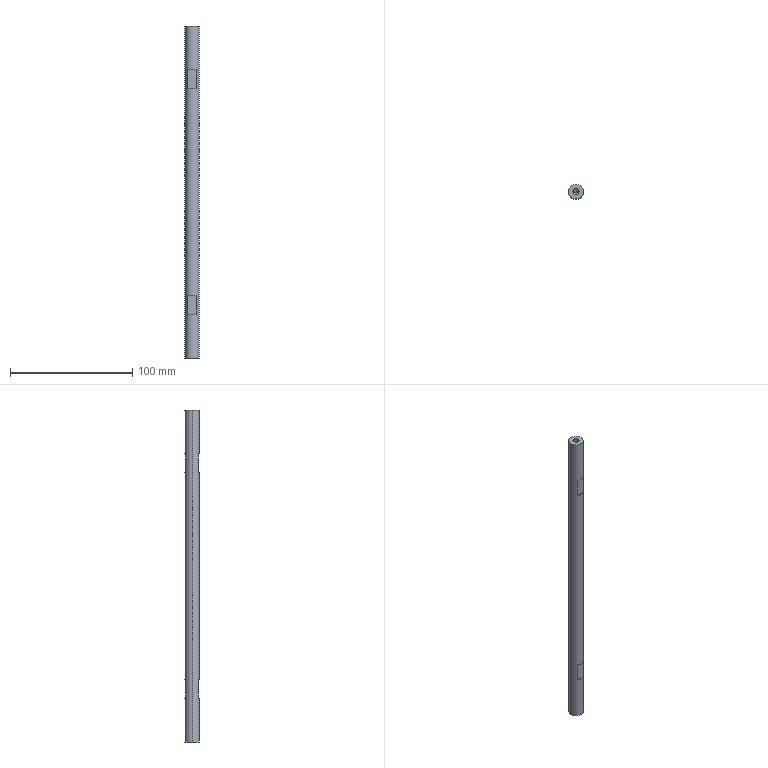Part | STEP file | GLSJ-10-30_default | 1 solid | 24 faces | box 12 x 12 x 272 mm | volume 29884 mm3 | plane 14 | cylinder 6 | cone 4 | commonest cylinder face diameters 5 x4 12 x2
STEP:
#1=CARTESIAN_POINT('',(0.,0.,0.));
#2=DIRECTION('',(0.,0.,1.));
#3=DIRECTION('',(1.,0.,0.));
#4=AXIS2_PLACEMENT_3D('',#1,#2,#3);
#5=CARTESIAN_POINT('',(-2.5,0.,-121.));
#6=VERTEX_POINT('',#5);
#7=CARTESIAN_POINT('',(-2.5,0.,-136.));
#8=VERTEX_POINT('',#7);
#9=CARTESIAN_POINT('',(-2.5,0.,-136.));
#10=DIRECTION('',(0.,0.,-1.));
#11=VECTOR('',#10,1.);
#12=LINE('',#9,#11);
#13=CARTESIAN_POINT('',(0.,0.,-136.));
#14=DIRECTION('',(0.,0.,-1.));
#15=DIRECTION('',(-1.,0.,0.));
#16=AXIS2_PLACEMENT_3D('',#13,#14,#15);
#17=CYLINDRICAL_SURFACE('',#16,2.5);
#18=CARTESIAN_POINT('',(6.283,0.));
#19=DIRECTION('',(0.,1.));
#20=VECTOR('',#19,1.);
#21=LINE('',#18,#20);
#22=(GEOMETRIC_REPRESENTATION_CONTEXT(2)PARAMETRIC_REPRESENTATION_CONTEXT()REPRESENTATION_CONTEXT('',''));
#23=DEFINITIONAL_REPRESENTATION('',(#21),#22);
#24=PCURVE('',#17,#23);
#25=CARTESIAN_POINT('',(0.,0.,-136.));
#26=DIRECTION('',(0.,0.,-1.));
#27=DIRECTION('',(-1.,0.,0.));
#28=AXIS2_PLACEMENT_3D('',#25,#26,#27);
#29=CYLINDRICAL_SURFACE('',#28,2.5);
#30=CARTESIAN_POINT('',(0.,0.));
#31=DIRECTION('',(0.,1.));
#32=VECTOR('',#31,1.);
#33=LINE('',#30,#32);
#34=(GEOMETRIC_REPRESENTATION_CONTEXT(2)PARAMETRIC_REPRESENTATION_CONTEXT()REPRESENTATION_CONTEXT('',''));
#35=DEFINITIONAL_REPRESENTATION('',(#33),#34);
#36=PCURVE('',#29,#35);
#37=SURFACE_CURVE('',#12,(#24,#36),.PCURVE_S1.);
#38=EDGE_CURVE('',#6,#8,#37,.T.);
#39=ORIENTED_EDGE('',*,*,#38,.T.);
#40=CARTESIAN_POINT('',(2.5,0.,-136.));
#41=VERTEX_POINT('',#40);
#42=CARTESIAN_POINT('',(0.,0.,-136.));
#43=DIRECTION('',(0.,0.,-1.));
#44=DIRECTION('',(-1.,0.,0.));
#45=AXIS2_PLACEMENT_3D('',#42,#43,#44);
#46=CIRCLE('',#45,2.5);
#47=CARTESIAN_POINT('',(0.,0.));
#48=DIRECTION('',(1.,0.));
#49=VECTOR('',#48,1.);
#50=LINE('',#47,#49);
#51=(GEOMETRIC_REPRESENTATION_CONTEXT(2)PARAMETRIC_REPRESENTATION_CONTEXT()REPRESENTATION_CONTEXT('',''));
#52=DEFINITIONAL_REPRESENTATION('',(#50),#51);
#53=PCURVE('',#17,#52);
#54=CARTESIAN_POINT('',(0.,0.,-136.));
#55=DIRECTION('',(0.,0.,1.));
#56=DIRECTION('',(1.,0.,0.));
#57=AXIS2_PLACEMENT_3D('',#54,#55,#56);
#58=PLANE('',#57);
#59=CARTESIAN_POINT('',(-2.5,0.));
#60=CARTESIAN_POINT('',(-2.5,4.33));
#61=CARTESIAN_POINT('',(1.25,2.165));
#62=CARTESIAN_POINT('',(5.,0.));
#63=CARTESIAN_POINT('',(1.25,-2.165));
#64=CARTESIAN_POINT('',(-2.5,-4.33));
#65=CARTESIAN_POINT('',(-2.5,0.));
#66=(BOUNDED_CURVE()B_SPLINE_CURVE(2,(#59,#60,#61,#62,#63,#64,#65),.UNSPECIFIED.,.T.,.F.)B_SPLINE_CURVE_WITH_KNOTS((1,2,2,2,2,1),(-2.094,0.,2.094,4.189,6.283,8.378),.UNSPECIFIED.)CURVE()GEOMETRIC_REPRESENTATION_ITEM()RATIONAL_B_SPLINE_CURVE((1.,0.5,1.,0.5,1.,0.5,1.))REPRESENTATION_ITEM(''));
#67=(GEOMETRIC_REPRESENTATION_CONTEXT(2)PARAMETRIC_REPRESENTATION_CONTEXT()REPRESENTATION_CONTEXT('',''));
#68=DEFINITIONAL_REPRESENTATION('',(#66),#67);
#69=PCURVE('',#58,#68);
#70=SURFACE_CURVE('',#46,(#53,#69),.PCURVE_S1.);
#71=EDGE_CURVE('',#41,#8,#70,.T.);
#72=ORIENTED_EDGE('',*,*,#71,.F.);
#73=CARTESIAN_POINT('',(2.5,0.,-121.));
#74=VERTEX_POINT('',#73);
#75=CARTESIAN_POINT('',(2.5,0.,-136.));
#76=DIRECTION('',(0.,0.,-1.));
#77=VECTOR('',#76,1.);
#78=LINE('',#75,#77);
#79=CARTESIAN_POINT('',(3.142,0.));
#80=DIRECTION('',(0.,1.));
#81=VECTOR('',#80,1.);
#82=LINE('',#79,#81);
#83=(GEOMETRIC_REPRESENTATION_CONTEXT(2)PARAMETRIC_REPRESENTATION_CONTEXT()REPRESENTATION_CONTEXT('',''));
#84=DEFINITIONAL_REPRESENTATION('',(#82),#83);
#85=PCURVE('',#17,#84);
#86=CARTESIAN_POINT('',(3.142,0.));
#87=DIRECTION('',(0.,1.));
#88=VECTOR('',#87,1.);
#89=LINE('',#86,#88);
#90=(GEOMETRIC_REPRESENTATION_CONTEXT(2)PARAMETRIC_REPRESENTATION_CONTEXT()REPRESENTATION_CONTEXT('',''));
#91=DEFINITIONAL_REPRESENTATION('',(#89),#90);
#92=PCURVE('',#29,#91);
#93=SURFACE_CURVE('',#78,(#85,#92),.PCURVE_S1.);
#94=EDGE_CURVE('',#74,#41,#93,.T.);
#95=ORIENTED_EDGE('',*,*,#94,.F.);
#96=CARTESIAN_POINT('',(0.,0.,-121.));
#97=DIRECTION('',(0.,0.,-1.));
#98=DIRECTION('',(-1.,0.,0.));
#99=AXIS2_PLACEMENT_3D('',#96,#97,#98);
#100=CIRCLE('',#99,2.5);
#101=CARTESIAN_POINT('',(0.,-15.));
#102=DIRECTION('',(1.,0.));
#103=VECTOR('',#102,1.);
#104=LINE('',#101,#103);
#105=(GEOMETRIC_REPRESENTATION_CONTEXT(2)PARAMETRIC_REPRESENTATION_CONTEXT()REPRESENTATION_CONTEXT('',''));
#106=DEFINITIONAL_REPRESENTATION('',(#104),#105);
#107=PCURVE('',#17,#106);
#108=CARTESIAN_POINT('',(0.,0.,-121.));
#109=DIRECTION('',(0.,0.,-1.));
#110=DIRECTION('',(-1.,0.,0.));
#111=AXIS2_PLACEMENT_3D('',#108,#109,#110);
#112=CONICAL_SURFACE('',#111,2.5,1.03);
#113=CARTESIAN_POINT('',(0.,0.));
#114=DIRECTION('',(1.,0.));
#115=VECTOR('',#114,1.);
#116=LINE('',#113,#115);
#117=(GEOMETRIC_REPRESENTATION_CONTEXT(2)PARAMETRIC_REPRESENTATION_CONTEXT()REPRESENTATION_CONTEXT('',''));
#118=DEFINITIONAL_REPRESENTATION('',(#116),#117);
#119=PCURVE('',#112,#118);
#120=SURFACE_CURVE('',#100,(#107,#119),.PCURVE_S1.);
#121=EDGE_CURVE('',#74,#6,#120,.T.);
#122=ORIENTED_EDGE('',*,*,#121,.T.);
#123=EDGE_LOOP('',(#39,#72,#95,#122));
#124=FACE_BOUND('',#123,.F.);
#125=ADVANCED_FACE('',(#124),#17,.F.);
#126=ORIENTED_EDGE('',*,*,#121,.F.);
#127=CARTESIAN_POINT('',(0.,0.,-119.498));
#128=VERTEX_POINT('',#127);
#129=CARTESIAN_POINT('',(2.5,0.,-121.));
#130=DIRECTION('',(0.8572,0.,-0.515));
#131=VECTOR('',#130,1.);
#132=LINE('',#129,#131);
#133=CARTESIAN_POINT('',(3.142,-1.502));
#134=CARTESIAN_POINT('',(3.142,-1.479));
#135=CARTESIAN_POINT('',(3.142,-1.434));
#136=CARTESIAN_POINT('',(3.142,-1.366));
#137=CARTESIAN_POINT('',(3.142,-1.297));
#138=CARTESIAN_POINT('',(3.142,-1.229));
#139=CARTESIAN_POINT('',(3.142,-1.161));
#140=CARTESIAN_POINT('',(3.142,-1.092));
#141=CARTESIAN_POINT('',(3.142,-1.024));
#142=CARTESIAN_POINT('',(3.142,-0.9559));
#143=CARTESIAN_POINT('',(3.142,-0.8876));
#144=CARTESIAN_POINT('',(3.142,-0.8194));
#145=CARTESIAN_POINT('',(3.142,-0.7511));
#146=CARTESIAN_POINT('',(3.142,-0.6828));
#147=CARTESIAN_POINT('',(3.142,-0.6145));
#148=CARTESIAN_POINT('',(3.142,-0.5462));
#149=CARTESIAN_POINT('',(3.142,-0.478));
#150=CARTESIAN_POINT('',(3.142,-0.4097));
#151=CARTESIAN_POINT('',(3.142,-0.3414));
#152=CARTESIAN_POINT('',(3.142,-0.2731));
#153=CARTESIAN_POINT('',(3.142,-0.2048));
#154=CARTESIAN_POINT('',(3.142,-0.1366));
#155=CARTESIAN_POINT('',(3.142,-0.06828));
#156=CARTESIAN_POINT('',(3.142,-0.02276));
#157=CARTESIAN_POINT('',(3.142,0.));
#158=B_SPLINE_CURVE_WITH_KNOTS('',3,(#133,#134,#135,#136,#137,#138,#139,#140,#141,#142,#143,#144,#145,#146,#147,#148,#149,#150,#151,#152,#153,#154,#155,#156,#157),.UNSPECIFIED.,.F.,.F.,(4,1,1,1,1,1,1,1,1,1,1,1,1,1,1,1,1,1,1,1,1,1,4),(-2.917,-2.784,-2.651,-2.519,-2.386,-2.254,-2.121,-1.989,-1.856,-1.723,-1.591,-1.458,-1.326,-1.193,-1.061,-0.928,-0.7954,-0.6629,-0.5303,-0.3977,-0.2651,-0.1326,0.),.QUASI_UNIFORM_KNOTS.);
#159=(GEOMETRIC_REPRESENTATION_CONTEXT(2)PARAMETRIC_REPRESENTATION_CONTEXT()REPRESENTATION_CONTEXT('',''));
#160=DEFINITIONAL_REPRESENTATION('',(#158),#159);
#161=PCURVE('',#112,#160);
#162=CARTESIAN_POINT('',(0.,0.,-121.));
#163=DIRECTION('',(0.,0.,-1.));
#164=DIRECTION('',(-1.,0.,0.));
#165=AXIS2_PLACEMENT_3D('',#162,#163,#164);
#166=CONICAL_SURFACE('',#165,2.5,1.03);
#167=CARTESIAN_POINT('',(3.142,-1.502));
#168=CARTESIAN_POINT('',(3.142,-1.479));
#169=CARTESIAN_POINT('',(3.142,-1.434));
#170=CARTESIAN_POINT('',(3.142,-1.366));
#171=CARTESIAN_POINT('',(3.142,-1.297));
#172=CARTESIAN_POINT('',(3.142,-1.229));
#173=CARTESIAN_POINT('',(3.142,-1.161));
#174=CARTESIAN_POINT('',(3.142,-1.092));
#175=CARTESIAN_POINT('',(3.142,-1.024));
#176=CARTESIAN_POINT('',(3.142,-0.9559));
#177=CARTESIAN_POINT('',(3.142,-0.8876));
#178=CARTESIAN_POINT('',(3.142,-0.8194));
#179=CARTESIAN_POINT('',(3.142,-0.7511));
#180=CARTESIAN_POINT('',(3.142,-0.6828));
#181=CARTESIAN_POINT('',(3.142,-0.6145));
#182=CARTESIAN_POINT('',(3.142,-0.5462));
#183=CARTESIAN_POINT('',(3.142,-0.478));
#184=CARTESIAN_POINT('',(3.142,-0.4097));
#185=CARTESIAN_POINT('',(3.142,-0.3414));
#186=CARTESIAN_POINT('',(3.142,-0.2731));
#187=CARTESIAN_POINT('',(3.142,-0.2048));
#188=CARTESIAN_POINT('',(3.142,-0.1366));
#189=CARTESIAN_POINT('',(3.142,-0.06828));
#190=CARTESIAN_POINT('',(3.142,-0.02276));
#191=CARTESIAN_POINT('',(3.142,0.));
#192=B_SPLINE_CURVE_WITH_KNOTS('',3,(#167,#168,#169,#170,#171,#172,#173,#174,#175,#176,#177,#178,#179,#180,#181,#182,#183,#184,#185,#186,#187,#188,#189,#190,#191),.UNSPECIFIED.,.F.,.F.,(4,1,1,1,1,1,1,1,1,1,1,1,1,1,1,1,1,1,1,1,1,1,4),(-2.917,-2.784,-2.651,-2.519,-2.386,-2.254,-2.121,-1.989,-1.856,-1.723,-1.591,-1.458,-1.326,-1.193,-1.061,-0.928,-0.7954,-0.6629,-0.5303,-0.3977,-0.2651,-0.1326,0.),.QUASI_UNIFORM_KNOTS.);
#193=(GEOMETRIC_REPRESENTATION_CONTEXT(2)PARAMETRIC_REPRESENTATION_CONTEXT()REPRESENTATION_CONTEXT('',''));
#194=DEFINITIONAL_REPRESENTATION('',(#192),#193);
#195=PCURVE('',#166,#194);
#196=SURFACE_CURVE('',#132,(#161,#195),.PCURVE_S1.);
#197=EDGE_CURVE('',#128,#74,#196,.T.);
#198=ORIENTED_EDGE('',*,*,#197,.F.);
#199=CARTESIAN_POINT('',(-2.5,0.,-121.));
#200=DIRECTION('',(-0.8572,0.,-0.515));
#201=VECTOR('',#200,1.);
#202=LINE('',#199,#201);
#203=CARTESIAN_POINT('',(6.283,0.));
#204=DIRECTION('',(0.,1.));
#205=VECTOR('',#204,1.);
#206=LINE('',#203,#205);
#207=(GEOMETRIC_REPRESENTATION_CONTEXT(2)PARAMETRIC_REPRESENTATION_CONTEXT()REPRESENTATION_CONTEXT('',''));
#208=DEFINITIONAL_REPRESENTATION('',(#206),#207);
#209=PCURVE('',#112,#208);
#210=CARTESIAN_POINT('',(0.,0.));
#211=DIRECTION('',(0.,1.));
#212=VECTOR('',#211,1.);
#213=LINE('',#210,#212);
#214=(GEOMETRIC_REPRESENTATION_CONTEXT(2)PARAMETRIC_REPRESENTATION_CONTEXT()REPRESENTATION_CONTEXT('',''));
#215=DEFINITIONAL_REPRESENTATION('',(#213),#214);
#216=PCURVE('',#166,#215);
#217=SURFACE_CURVE('',#202,(#209,#216),.PCURVE_S1.);
#218=EDGE_CURVE('',#128,#6,#217,.T.);
#219=ORIENTED_EDGE('',*,*,#218,.T.);
#220=EDGE_LOOP('',(#126,#198,#219));
#221=FACE_BOUND('',#220,.F.);
#222=ADVANCED_FACE('',(#221),#112,.F.);
#223=CARTESIAN_POINT('',(2.5,0.,121.));
#224=VERTEX_POINT('',#223);
#225=CARTESIAN_POINT('',(2.5,0.,136.));
#226=VERTEX_POINT('',#225);
#227=CARTESIAN_POINT('',(2.5,0.,136.));
#228=DIRECTION('',(0.,0.,1.));
#229=VECTOR('',#228,1.);
#230=LINE('',#227,#229);
#231=CARTESIAN_POINT('',(0.,0.,136.));
#232=DIRECTION('',(0.,0.,1.));
#233=DIRECTION('',(1.,0.,0.));
#234=AXIS2_PLACEMENT_3D('',#231,#232,#233);
#235=CYLINDRICAL_SURFACE('',#234,2.5);
#236=CARTESIAN_POINT('',(6.283,0.));
#237=DIRECTION('',(0.,1.));
#238=VECTOR('',#237,1.);
#239=LINE('',#236,#238);
#240=(GEOMETRIC_REPRESENTATION_CONTEXT(2)PARAMETRIC_REPRESENTATION_CONTEXT()REPRESENTATION_CONTEXT('',''));
#241=DEFINITIONAL_REPRESENTATION('',(#239),#240);
#242=PCURVE('',#235,#241);
#243=CARTESIAN_POINT('',(0.,0.,136.));
#244=DIRECTION('',(0.,0.,1.));
#245=DIRECTION('',(1.,0.,0.));
#246=AXIS2_PLACEMENT_3D('',#243,#244,#245);
#247=CYLINDRICAL_SURFACE('',#246,2.5);
#248=CARTESIAN_POINT('',(0.,0.));
#249=DIRECTION('',(0.,1.));
#250=VECTOR('',#249,1.);
#251=LINE('',#248,#250);
#252=(GEOMETRIC_REPRESENTATION_CONTEXT(2)PARAMETRIC_REPRESENTATION_CONTEXT()REPRESENTATION_CONTEXT('',''));
#253=DEFINITIONAL_REPRESENTATION('',(#251),#252);
#254=PCURVE('',#247,#253);
#255=SURFACE_CURVE('',#230,(#242,#254),.PCURVE_S1.);
#256=EDGE_CURVE('',#224,#226,#255,.T.);
#257=ORIENTED_EDGE('',*,*,#256,.T.);
#258=CARTESIAN_POINT('',(-2.5,0.,136.));
#259=VERTEX_POINT('',#258);
#260=CARTESIAN_POINT('',(0.,0.,136.));
#261=DIRECTION('',(0.,0.,1.));
#262=DIRECTION('',(1.,0.,0.));
#263=AXIS2_PLACEMENT_3D('',#260,#261,#262);
#264=CIRCLE('',#263,2.5);
#265=CARTESIAN_POINT('',(0.,0.));
#266=DIRECTION('',(1.,0.));
#267=VECTOR('',#266,1.);
#268=LINE('',#265,#267);
#269=(GEOMETRIC_REPRESENTATION_CONTEXT(2)PARAMETRIC_REPRESENTATION_CONTEXT()REPRESENTATION_CONTEXT('',''));
#270=DEFINITIONAL_REPRESENTATION('',(#268),#269);
#271=PCURVE('',#235,#270);
#272=CARTESIAN_POINT('',(0.,0.,136.));
#273=DIRECTION('',(0.,0.,1.));
#274=DIRECTION('',(1.,0.,0.));
#275=AXIS2_PLACEMENT_3D('',#272,#273,#274);
#276=PLANE('',#275);
#277=CARTESIAN_POINT('',(0.,0.));
#278=DIRECTION('',(1.,0.));
#279=AXIS2_PLACEMENT_2D('',#277,#278);
#280=CIRCLE('',#279,2.5);
#281=(GEOMETRIC_REPRESENTATION_CONTEXT(2)PARAMETRIC_REPRESENTATION_CONTEXT()REPRESENTATION_CONTEXT('',''));
#282=DEFINITIONAL_REPRESENTATION('',(#280),#281);
#283=PCURVE('',#276,#282);
#284=SURFACE_CURVE('',#264,(#271,#283),.PCURVE_S1.);
#285=EDGE_CURVE('',#259,#226,#284,.T.);
#286=ORIENTED_EDGE('',*,*,#285,.F.);
#287=CARTESIAN_POINT('',(-2.5,0.,121.));
#288=VERTEX_POINT('',#287);
#289=CARTESIAN_POINT('',(-2.5,0.,136.));
#290=DIRECTION('',(0.,0.,1.));
#291=VECTOR('',#290,1.);
#292=LINE('',#289,#291);
#293=CARTESIAN_POINT('',(3.142,0.));
#294=DIRECTION('',(0.,1.));
#295=VECTOR('',#294,1.);
#296=LINE('',#293,#295);
#297=(GEOMETRIC_REPRESENTATION_CONTEXT(2)PARAMETRIC_REPRESENTATION_CONTEXT()REPRESENTATION_CONTEXT('',''));
#298=DEFINITIONAL_REPRESENTATION('',(#296),#297);
#299=PCURVE('',#235,#298);
#300=CARTESIAN_POINT('',(3.142,0.));
#301=DIRECTION('',(0.,1.));
#302=VECTOR('',#301,1.);
#303=LINE('',#300,#302);
#304=(GEOMETRIC_REPRESENTATION_CONTEXT(2)PARAMETRIC_REPRESENTATION_CONTEXT()REPRESENTATION_CONTEXT('',''));
#305=DEFINITIONAL_REPRESENTATION('',(#303),#304);
#306=PCURVE('',#247,#305);
#307=SURFACE_CURVE('',#292,(#299,#306),.PCURVE_S1.);
#308=EDGE_CURVE('',#288,#259,#307,.T.);
#309=ORIENTED_EDGE('',*,*,#308,.F.);
#310=CARTESIAN_POINT('',(0.,0.,121.));
#311=DIRECTION('',(0.,0.,1.));
#312=DIRECTION('',(1.,0.,0.));
#313=AXIS2_PLACEMENT_3D('',#310,#311,#312);
#314=CIRCLE('',#313,2.5);
#315=CARTESIAN_POINT('',(0.,-15.));
#316=DIRECTION('',(1.,0.));
#317=VECTOR('',#316,1.);
#318=LINE('',#315,#317);
#319=(GEOMETRIC_REPRESENTATION_CONTEXT(2)PARAMETRIC_REPRESENTATION_CONTEXT()REPRESENTATION_CONTEXT('',''));
#320=DEFINITIONAL_REPRESENTATION('',(#318),#319);
#321=PCURVE('',#235,#320);
#322=CARTESIAN_POINT('',(0.,0.,121.));
#323=DIRECTION('',(0.,0.,1.));
#324=DIRECTION('',(1.,0.,0.));
#325=AXIS2_PLACEMENT_3D('',#322,#323,#324);
#326=CONICAL_SURFACE('',#325,2.5,1.03);
#327=CARTESIAN_POINT('',(0.,0.));
#328=DIRECTION('',(1.,0.));
#329=VECTOR('',#328,1.);
#330=LINE('',#327,#329);
#331=(GEOMETRIC_REPRESENTATION_CONTEXT(2)PARAMETRIC_REPRESENTATION_CONTEXT()REPRESENTATION_CONTEXT('',''));
#332=DEFINITIONAL_REPRESENTATION('',(#330),#331);
#333=PCURVE('',#326,#332);
#334=SURFACE_CURVE('',#314,(#321,#333),.PCURVE_S1.);
#335=EDGE_CURVE('',#288,#224,#334,.T.);
#336=ORIENTED_EDGE('',*,*,#335,.T.);
#337=EDGE_LOOP('',(#257,#286,#309,#336));
#338=FACE_BOUND('',#337,.F.);
#339=ADVANCED_FACE('',(#338),#235,.F.);
#340=ORIENTED_EDGE('',*,*,#335,.F.);
#341=CARTESIAN_POINT('',(0.,0.,119.498));
#342=VERTEX_POINT('',#341);
#343=CARTESIAN_POINT('',(-2.5,0.,121.));
#344=DIRECTION('',(-0.8572,0.,0.515));
#345=VECTOR('',#344,1.);
#346=LINE('',#343,#345);
#347=CARTESIAN_POINT('',(3.142,0.));
#348=DIRECTION('',(0.,1.));
#349=VECTOR('',#348,1.);
#350=LINE('',#347,#349);
#351=(GEOMETRIC_REPRESENTATION_CONTEXT(2)PARAMETRIC_REPRESENTATION_CONTEXT()REPRESENTATION_CONTEXT('',''));
#352=DEFINITIONAL_REPRESENTATION('',(#350),#351);
#353=PCURVE('',#326,#352);
#354=CARTESIAN_POINT('',(0.,0.,121.));
#355=DIRECTION('',(0.,0.,1.));
#356=DIRECTION('',(1.,0.,0.));
#357=AXIS2_PLACEMENT_3D('',#354,#355,#356);
#358=CONICAL_SURFACE('',#357,2.5,1.03);
#359=CARTESIAN_POINT('',(3.142,0.));
#360=DIRECTION('',(0.,1.));
#361=VECTOR('',#360,1.);
#362=LINE('',#359,#361);
#363=(GEOMETRIC_REPRESENTATION_CONTEXT(2)PARAMETRIC_REPRESENTATION_CONTEXT()REPRESENTATION_CONTEXT('',''));
#364=DEFINITIONAL_REPRESENTATION('',(#362),#363);
#365=PCURVE('',#358,#364);
#366=SURFACE_CURVE('',#346,(#353,#365),.PCURVE_S1.);
#367=EDGE_CURVE('',#342,#288,#366,.T.);
#368=ORIENTED_EDGE('',*,*,#367,.F.);
#369=CARTESIAN_POINT('',(2.5,0.,121.));
#370=DIRECTION('',(0.8572,0.,0.515));
#371=VECTOR('',#370,1.);
#372=LINE('',#369,#371);
#373=CARTESIAN_POINT('',(6.283,-1.502));
#374=CARTESIAN_POINT('',(6.283,-1.479));
#375=CARTESIAN_POINT('',(6.283,-1.434));
#376=CARTESIAN_POINT('',(6.283,-1.366));
#377=CARTESIAN_POINT('',(6.283,-1.297));
#378=CARTESIAN_POINT('',(6.283,-1.229));
#379=CARTESIAN_POINT('',(6.283,-1.161));
#380=CARTESIAN_POINT('',(6.283,-1.092));
#381=CARTESIAN_POINT('',(6.283,-1.024));
#382=CARTESIAN_POINT('',(6.283,-0.9559));
#383=CARTESIAN_POINT('',(6.283,-0.8876));
#384=CARTESIAN_POINT('',(6.283,-0.8194));
#385=CARTESIAN_POINT('',(6.283,-0.7511));
#386=CARTESIAN_POINT('',(6.283,-0.6828));
#387=CARTESIAN_POINT('',(6.283,-0.6145));
#388=CARTESIAN_POINT('',(6.283,-0.5462));
#389=CARTESIAN_POINT('',(6.283,-0.478));
#390=CARTESIAN_POINT('',(6.283,-0.4097));
#391=CARTESIAN_POINT('',(6.283,-0.3414));
#392=CARTESIAN_POINT('',(6.283,-0.2731));
#393=CARTESIAN_POINT('',(6.283,-0.2048));
#394=CARTESIAN_POINT('',(6.283,-0.1366));
#395=CARTESIAN_POINT('',(6.283,-0.06828));
#396=CARTESIAN_POINT('',(6.283,-0.02276));
#397=CARTESIAN_POINT('',(6.283,0.));
#398=B_SPLINE_CURVE_WITH_KNOTS('',3,(#373,#374,#375,#376,#377,#378,#379,#380,#381,#382,#383,#384,#385,#386,#387,#388,#389,#390,#391,#392,#393,#394,#395,#396,#397),.UNSPECIFIED.,.F.,.F.,(4,1,1,1,1,1,1,1,1,1,1,1,1,1,1,1,1,1,1,1,1,1,4),(-2.917,-2.784,-2.651,-2.519,-2.386,-2.254,-2.121,-1.989,-1.856,-1.723,-1.591,-1.458,-1.326,-1.193,-1.061,-0.928,-0.7954,-0.6629,-0.5303,-0.3977,-0.2651,-0.1326,0.),.QUASI_UNIFORM_KNOTS.);
#399=(GEOMETRIC_REPRESENTATION_CONTEXT(2)PARAMETRIC_REPRESENTATION_CONTEXT()REPRESENTATION_CONTEXT('',''));
#400=DEFINITIONAL_REPRESENTATION('',(#398),#399);
#401=PCURVE('',#326,#400);
#402=CARTESIAN_POINT('',(0.,-1.502));
#403=CARTESIAN_POINT('',(0.,-1.479));
#404=CARTESIAN_POINT('',(0.,-1.434));
#405=CARTESIAN_POINT('',(0.,-1.366));
#406=CARTESIAN_POINT('',(0.,-1.297));
#407=CARTESIAN_POINT('',(0.,-1.229));
#408=CARTESIAN_POINT('',(0.,-1.161));
#409=CARTESIAN_POINT('',(0.,-1.092));
#410=CARTESIAN_POINT('',(0.,-1.024));
#411=CARTESIAN_POINT('',(0.,-0.9559));
#412=CARTESIAN_POINT('',(0.,-0.8876));
#413=CARTESIAN_POINT('',(0.,-0.8194));
#414=CARTESIAN_POINT('',(0.,-0.7511));
#415=CARTESIAN_POINT('',(0.,-0.6828));
#416=CARTESIAN_POINT('',(0.,-0.6145));
#417=CARTESIAN_POINT('',(0.,-0.5462));
#418=CARTESIAN_POINT('',(0.,-0.478));
#419=CARTESIAN_POINT('',(0.,-0.4097));
#420=CARTESIAN_POINT('',(0.,-0.3414));
#421=CARTESIAN_POINT('',(0.,-0.2731));
#422=CARTESIAN_POINT('',(0.,-0.2048));
#423=CARTESIAN_POINT('',(0.,-0.1366));
#424=CARTESIAN_POINT('',(0.,-0.06828));
#425=CARTESIAN_POINT('',(0.,-0.02276));
#426=CARTESIAN_POINT('',(0.,0.));
#427=B_SPLINE_CURVE_WITH_KNOTS('',3,(#402,#403,#404,#405,#406,#407,#408,#409,#410,#411,#412,#413,#414,#415,#416,#417,#418,#419,#420,#421,#422,#423,#424,#425,#426),.UNSPECIFIED.,.F.,.F.,(4,1,1,1,1,1,1,1,1,1,1,1,1,1,1,1,1,1,1,1,1,1,4),(-2.917,-2.784,-2.651,-2.519,-2.386,-2.254,-2.121,-1.989,-1.856,-1.723,-1.591,-1.458,-1.326,-1.193,-1.061,-0.928,-0.7954,-0.6629,-0.5303,-0.3977,-0.2651,-0.1326,0.),.QUASI_UNIFORM_KNOTS.);
#428=(GEOMETRIC_REPRESENTATION_CONTEXT(2)PARAMETRIC_REPRESENTATION_CONTEXT()REPRESENTATION_CONTEXT('',''));
#429=DEFINITIONAL_REPRESENTATION('',(#427),#428);
#430=PCURVE('',#358,#429);
#431=SURFACE_CURVE('',#372,(#401,#430),.PCURVE_S1.);
#432=EDGE_CURVE('',#342,#224,#431,.T.);
#433=ORIENTED_EDGE('',*,*,#432,.T.);
#434=EDGE_LOOP('',(#340,#368,#433));
#435=FACE_BOUND('',#434,.F.);
#436=ADVANCED_FACE('',(#435),#326,.F.);
#437=CARTESIAN_POINT('',(3.317,5.,100.));
#438=VERTEX_POINT('',#437);
#439=CARTESIAN_POINT('',(-3.317,5.,100.));
#440=VERTEX_POINT('',#439);
#441=CARTESIAN_POINT('',(0.,0.,100.));
#442=DIRECTION('',(0.,0.,1.));
#443=DIRECTION('',(1.,0.,0.));
#444=AXIS2_PLACEMENT_3D('',#441,#442,#443);
#445=CIRCLE('',#444,6.);
#446=CARTESIAN_POINT('',(0.,0.,136.));
#447=DIRECTION('',(0.,0.,-1.));
#448=DIRECTION('',(-1.,0.,0.));
#449=AXIS2_PLACEMENT_3D('',#446,#447,#448);
#450=CYLINDRICAL_SURFACE('',#449,6.);
#451=CARTESIAN_POINT('',(3.142,36.));
#452=DIRECTION('',(-1.,0.));
#453=VECTOR('',#452,1.);
#454=LINE('',#451,#453);
#455=(GEOMETRIC_REPRESENTATION_CONTEXT(2)PARAMETRIC_REPRESENTATION_CONTEXT()REPRESENTATION_CONTEXT('',''));
#456=DEFINITIONAL_REPRESENTATION('',(#454),#455);
#457=PCURVE('',#450,#456);
#458=CARTESIAN_POINT('',(-10.,7.,100.));
#459=DIRECTION('',(0.,0.,1.));
#460=DIRECTION('',(1.,0.,0.));
#461=AXIS2_PLACEMENT_3D('',#458,#459,#460);
#462=PLANE('',#461);
#463=CARTESIAN_POINT('',(10.,-7.));
#464=DIRECTION('',(1.,0.));
#465=AXIS2_PLACEMENT_2D('',#463,#464);
#466=CIRCLE('',#465,6.);
#467=(GEOMETRIC_REPRESENTATION_CONTEXT(2)PARAMETRIC_REPRESENTATION_CONTEXT()REPRESENTATION_CONTEXT('',''));
#468=DEFINITIONAL_REPRESENTATION('',(#466),#467);
#469=PCURVE('',#462,#468);
#470=SURFACE_CURVE('',#445,(#457,#469),.PCURVE_S1.);
#471=EDGE_CURVE('',#438,#440,#470,.T.);
#472=ORIENTED_EDGE('',*,*,#471,.T.);
#473=CARTESIAN_POINT('',(-3.317,5.,85.));
#474=VERTEX_POINT('',#473);
#475=CARTESIAN_POINT('',(-3.317,5.,136.));
#476=DIRECTION('',(0.,0.,-1.));
#477=VECTOR('',#476,1.);
#478=LINE('',#475,#477);
#479=CARTESIAN_POINT('',(0.9851,0.));
#480=DIRECTION('',(0.,1.));
#481=VECTOR('',#480,1.);
#482=LINE('',#479,#481);
#483=(GEOMETRIC_REPRESENTATION_CONTEXT(2)PARAMETRIC_REPRESENTATION_CONTEXT()REPRESENTATION_CONTEXT('',''));
#484=DEFINITIONAL_REPRESENTATION('',(#482),#483);
#485=PCURVE('',#450,#484);
#486=CARTESIAN_POINT('',(-10.,5.,100.));
#487=DIRECTION('',(0.,-1.,0.));
#488=DIRECTION('',(0.,0.,-1.));
#489=AXIS2_PLACEMENT_3D('',#486,#487,#488);
#490=PLANE('',#489);
#491=CARTESIAN_POINT('',(-36.,6.683));
#492=DIRECTION('',(1.,0.));
#493=VECTOR('',#492,1.);
#494=LINE('',#491,#493);
#495=(GEOMETRIC_REPRESENTATION_CONTEXT(2)PARAMETRIC_REPRESENTATION_CONTEXT()REPRESENTATION_CONTEXT('',''));
#496=DEFINITIONAL_REPRESENTATION('',(#494),#495);
#497=PCURVE('',#490,#496);
#498=SURFACE_CURVE('',#478,(#485,#497),.PCURVE_S1.);
#499=EDGE_CURVE('',#440,#474,#498,.T.);
#500=ORIENTED_EDGE('',*,*,#499,.T.);
#501=CARTESIAN_POINT('',(3.317,5.,85.));
#502=VERTEX_POINT('',#501);
#503=CARTESIAN_POINT('',(0.,0.,85.));
#504=DIRECTION('',(0.,0.,-1.));
#505=DIRECTION('',(-1.,0.,0.));
#506=AXIS2_PLACEMENT_3D('',#503,#504,#505);
#507=CIRCLE('',#506,6.);
#508=CARTESIAN_POINT('',(0.,51.));
#509=DIRECTION('',(1.,0.));
#510=VECTOR('',#509,1.);
#511=LINE('',#508,#510);
#512=(GEOMETRIC_REPRESENTATION_CONTEXT(2)PARAMETRIC_REPRESENTATION_CONTEXT()REPRESENTATION_CONTEXT('',''));
#513=DEFINITIONAL_REPRESENTATION('',(#511),#512);
#514=PCURVE('',#450,#513);
#515=CARTESIAN_POINT('',(-10.,7.,85.));
#516=DIRECTION('',(0.,0.,-1.));
#517=DIRECTION('',(-1.,0.,0.));
#518=AXIS2_PLACEMENT_3D('',#515,#516,#517);
#519=PLANE('',#518);
#520=CARTESIAN_POINT('',(-10.,-7.));
#521=DIRECTION('',(1.,0.));
#522=AXIS2_PLACEMENT_2D('',#520,#521);
#523=CIRCLE('',#522,6.);
#524=(GEOMETRIC_REPRESENTATION_CONTEXT(2)PARAMETRIC_REPRESENTATION_CONTEXT()REPRESENTATION_CONTEXT('',''));
#525=DEFINITIONAL_REPRESENTATION('',(#523),#524);
#526=PCURVE('',#519,#525);
#527=SURFACE_CURVE('',#507,(#514,#526),.PCURVE_S1.);
#528=EDGE_CURVE('',#474,#502,#527,.T.);
#529=ORIENTED_EDGE('',*,*,#528,.T.);
#530=CARTESIAN_POINT('',(3.317,5.,136.));
#531=DIRECTION('',(0.,0.,1.));
#532=VECTOR('',#531,1.);
#533=LINE('',#530,#532);
#534=CARTESIAN_POINT('',(2.156,0.));
#535=DIRECTION('',(0.,-1.));
#536=VECTOR('',#535,1.);
#537=LINE('',#534,#536);
#538=(GEOMETRIC_REPRESENTATION_CONTEXT(2)PARAMETRIC_REPRESENTATION_CONTEXT()REPRESENTATION_CONTEXT('',''));
#539=DEFINITIONAL_REPRESENTATION('',(#537),#538);
#540=PCURVE('',#450,#539);
#541=CARTESIAN_POINT('',(-36.,13.317));
#542=DIRECTION('',(-1.,0.));
#543=VECTOR('',#542,1.);
#544=LINE('',#541,#543);
#545=(GEOMETRIC_REPRESENTATION_CONTEXT(2)PARAMETRIC_REPRESENTATION_CONTEXT()REPRESENTATION_CONTEXT('',''));
#546=DEFINITIONAL_REPRESENTATION('',(#544),#545);
#547=PCURVE('',#490,#546);
#548=SURFACE_CURVE('',#533,(#540,#547),.PCURVE_S1.);
#549=EDGE_CURVE('',#502,#438,#548,.T.);
#550=ORIENTED_EDGE('',*,*,#549,.T.);
#551=EDGE_LOOP('',(#472,#500,#529,#550));
#552=FACE_BOUND('',#551,.T.);
#553=CARTESIAN_POINT('',(-3.317,5.,-85.));
#554=VERTEX_POINT('',#553);
#555=CARTESIAN_POINT('',(-3.317,5.,-100.));
#556=VERTEX_POINT('',#555);
#557=CARTESIAN_POINT('',(-3.317,5.,136.));
#558=DIRECTION('',(0.,0.,-1.));
#559=VECTOR('',#558,1.);
#560=LINE('',#557,#559);
#561=CARTESIAN_POINT('',(0.9851,0.));
#562=DIRECTION('',(0.,1.));
#563=VECTOR('',#562,1.);
#564=LINE('',#561,#563);
#565=(GEOMETRIC_REPRESENTATION_CONTEXT(2)PARAMETRIC_REPRESENTATION_CONTEXT()REPRESENTATION_CONTEXT('',''));
#566=DEFINITIONAL_REPRESENTATION('',(#564),#565);
#567=PCURVE('',#450,#566);
#568=CARTESIAN_POINT('',(-10.,5.,-100.));
#569=DIRECTION('',(0.,-1.,0.));
#570=DIRECTION('',(0.,0.,-1.));
#571=AXIS2_PLACEMENT_3D('',#568,#569,#570);
#572=PLANE('',#571);
#573=CARTESIAN_POINT('',(-236.,6.683));
#574=DIRECTION('',(1.,0.));
#575=VECTOR('',#574,1.);
#576=LINE('',#573,#575);
#577=(GEOMETRIC_REPRESENTATION_CONTEXT(2)PARAMETRIC_REPRESENTATION_CONTEXT()REPRESENTATION_CONTEXT('',''));
#578=DEFINITIONAL_REPRESENTATION('',(#576),#577);
#579=PCURVE('',#572,#578);
#580=SURFACE_CURVE('',#560,(#567,#579),.PCURVE_S1.);
#581=EDGE_CURVE('',#554,#556,#580,.T.);
#582=ORIENTED_EDGE('',*,*,#581,.T.);
#583=CARTESIAN_POINT('',(3.317,5.,-100.));
#584=VERTEX_POINT('',#583);
#585=CARTESIAN_POINT('',(0.,0.,-100.));
#586=DIRECTION('',(0.,0.,-1.));
#587=DIRECTION('',(-1.,0.,0.));
#588=AXIS2_PLACEMENT_3D('',#585,#586,#587);
#589=CIRCLE('',#588,6.);
#590=CARTESIAN_POINT('',(0.,236.));
#591=DIRECTION('',(1.,0.));
#592=VECTOR('',#591,1.);
#593=LINE('',#590,#592);
#594=(GEOMETRIC_REPRESENTATION_CONTEXT(2)PARAMETRIC_REPRESENTATION_CONTEXT()REPRESENTATION_CONTEXT('',''));
#595=DEFINITIONAL_REPRESENTATION('',(#593),#594);
#596=PCURVE('',#450,#595);
#597=CARTESIAN_POINT('',(-10.,7.,-100.));
#598=DIRECTION('',(0.,0.,-1.));
#599=DIRECTION('',(-1.,0.,0.));
#600=AXIS2_PLACEMENT_3D('',#597,#598,#599);
#601=PLANE('',#600);
#602=CARTESIAN_POINT('',(-10.,-7.));
#603=DIRECTION('',(1.,0.));
#604=AXIS2_PLACEMENT_2D('',#602,#603);
#605=CIRCLE('',#604,6.);
#606=(GEOMETRIC_REPRESENTATION_CONTEXT(2)PARAMETRIC_REPRESENTATION_CONTEXT()REPRESENTATION_CONTEXT('',''));
#607=DEFINITIONAL_REPRESENTATION('',(#605),#606);
#608=PCURVE('',#601,#607);
#609=SURFACE_CURVE('',#589,(#596,#608),.PCURVE_S1.);
#610=EDGE_CURVE('',#556,#584,#609,.T.);
#611=ORIENTED_EDGE('',*,*,#610,.T.);
#612=CARTESIAN_POINT('',(3.317,5.,-85.));
#613=VERTEX_POINT('',#612);
#614=CARTESIAN_POINT('',(3.317,5.,136.));
#615=DIRECTION('',(0.,0.,1.));
#616=VECTOR('',#615,1.);
#617=LINE('',#614,#616);
#618=CARTESIAN_POINT('',(2.156,0.));
#619=DIRECTION('',(0.,-1.));
#620=VECTOR('',#619,1.);
#621=LINE('',#618,#620);
#622=(GEOMETRIC_REPRESENTATION_CONTEXT(2)PARAMETRIC_REPRESENTATION_CONTEXT()REPRESENTATION_CONTEXT('',''));
#623=DEFINITIONAL_REPRESENTATION('',(#621),#622);
#624=PCURVE('',#450,#623);
#625=CARTESIAN_POINT('',(-236.,13.317));
#626=DIRECTION('',(-1.,0.));
#627=VECTOR('',#626,1.);
#628=LINE('',#625,#627);
#629=(GEOMETRIC_REPRESENTATION_CONTEXT(2)PARAMETRIC_REPRESENTATION_CONTEXT()REPRESENTATION_CONTEXT('',''));
#630=DEFINITIONAL_REPRESENTATION('',(#628),#629);
#631=PCURVE('',#572,#630);
#632=SURFACE_CURVE('',#617,(#624,#631),.PCURVE_S1.);
#633=EDGE_CURVE('',#584,#613,#632,.T.);
#634=ORIENTED_EDGE('',*,*,#633,.T.);
#635=CARTESIAN_POINT('',(0.,0.,-85.));
#636=DIRECTION('',(0.,0.,1.));
#637=DIRECTION('',(1.,0.,0.));
#638=AXIS2_PLACEMENT_3D('',#635,#636,#637);
#639=CIRCLE('',#638,6.);
#640=CARTESIAN_POINT('',(3.142,221.));
#641=DIRECTION('',(-1.,0.));
#642=VECTOR('',#641,1.);
#643=LINE('',#640,#642);
#644=(GEOMETRIC_REPRESENTATION_CONTEXT(2)PARAMETRIC_REPRESENTATION_CONTEXT()REPRESENTATION_CONTEXT('',''));
#645=DEFINITIONAL_REPRESENTATION('',(#643),#644);
#646=PCURVE('',#450,#645);
#647=CARTESIAN_POINT('',(-10.,7.,-85.));
#648=DIRECTION('',(0.,0.,1.));
#649=DIRECTION('',(1.,0.,0.));
#650=AXIS2_PLACEMENT_3D('',#647,#648,#649);
#651=PLANE('',#650);
#652=CARTESIAN_POINT('',(10.,-7.));
#653=DIRECTION('',(1.,0.));
#654=AXIS2_PLACEMENT_2D('',#652,#653);
#655=CIRCLE('',#654,6.);
#656=(GEOMETRIC_REPRESENTATION_CONTEXT(2)PARAMETRIC_REPRESENTATION_CONTEXT()REPRESENTATION_CONTEXT('',''));
#657=DEFINITIONAL_REPRESENTATION('',(#655),#656);
#658=PCURVE('',#651,#657);
#659=SURFACE_CURVE('',#639,(#646,#658),.PCURVE_S1.);
#660=EDGE_CURVE('',#613,#554,#659,.T.);
#661=ORIENTED_EDGE('',*,*,#660,.T.);
#662=EDGE_LOOP('',(#582,#611,#634,#661));
#663=FACE_BOUND('',#662,.T.);
#664=CARTESIAN_POINT('',(6.,0.,136.));
#665=VERTEX_POINT('',#664);
#666=CARTESIAN_POINT('',(-6.,0.,136.));
#667=VERTEX_POINT('',#666);
#668=CARTESIAN_POINT('',(0.,0.,136.));
#669=DIRECTION('',(0.,0.,1.));
#670=DIRECTION('',(1.,0.,0.));
#671=AXIS2_PLACEMENT_3D('',#668,#669,#670);
#672=CIRCLE('',#671,6.);
#673=CARTESIAN_POINT('',(3.142,0.));
#674=DIRECTION('',(-1.,0.));
#675=VECTOR('',#674,1.);
#676=LINE('',#673,#675);
#677=(GEOMETRIC_REPRESENTATION_CONTEXT(2)PARAMETRIC_REPRESENTATION_CONTEXT()REPRESENTATION_CONTEXT('',''));
#678=DEFINITIONAL_REPRESENTATION('',(#676),#677);
#679=PCURVE('',#450,#678);
#680=CARTESIAN_POINT('',(0.,0.));
#681=DIRECTION('',(1.,0.));
#682=AXIS2_PLACEMENT_2D('',#680,#681);
#683=CIRCLE('',#682,6.);
#684=(GEOMETRIC_REPRESENTATION_CONTEXT(2)PARAMETRIC_REPRESENTATION_CONTEXT()REPRESENTATION_CONTEXT('',''));
#685=DEFINITIONAL_REPRESENTATION('',(#683),#684);
#686=PCURVE('',#276,#685);
#687=SURFACE_CURVE('',#672,(#679,#686),.PCURVE_S1.);
#688=EDGE_CURVE('',#665,#667,#687,.T.);
#689=ORIENTED_EDGE('',*,*,#688,.F.);
#690=CARTESIAN_POINT('',(6.,0.,-136.));
#691=VERTEX_POINT('',#690);
#692=CARTESIAN_POINT('',(6.,0.,136.));
#693=DIRECTION('',(0.,0.,-1.));
#694=VECTOR('',#693,1.);
#695=LINE('',#692,#694);
#696=CARTESIAN_POINT('',(3.142,0.));
#697=DIRECTION('',(0.,1.));
#698=VECTOR('',#697,1.);
#699=LINE('',#696,#698);
#700=(GEOMETRIC_REPRESENTATION_CONTEXT(2)PARAMETRIC_REPRESENTATION_CONTEXT()REPRESENTATION_CONTEXT('',''));
#701=DEFINITIONAL_REPRESENTATION('',(#699),#700);
#702=PCURVE('',#450,#701);
#703=CARTESIAN_POINT('',(0.,0.,136.));
#704=DIRECTION('',(0.,0.,-1.));
#705=DIRECTION('',(-1.,0.,0.));
#706=AXIS2_PLACEMENT_3D('',#703,#704,#705);
#707=CYLINDRICAL_SURFACE('',#706,6.);
#708=CARTESIAN_POINT('',(3.142,0.));
#709=DIRECTION('',(0.,1.));
#710=VECTOR('',#709,1.);
#711=LINE('',#708,#710);
#712=(GEOMETRIC_REPRESENTATION_CONTEXT(2)PARAMETRIC_REPRESENTATION_CONTEXT()REPRESENTATION_CONTEXT('',''));
#713=DEFINITIONAL_REPRESENTATION('',(#711),#712);
#714=PCURVE('',#707,#713);
#715=SURFACE_CURVE('',#695,(#702,#714),.PCURVE_S1.);
#716=EDGE_CURVE('',#665,#691,#715,.T.);
#717=ORIENTED_EDGE('',*,*,#716,.T.);
#718=CARTESIAN_POINT('',(-6.,0.,-136.));
#719=VERTEX_POINT('',#718);
#720=CARTESIAN_POINT('',(0.,0.,-136.));
#721=DIRECTION('',(0.,0.,1.));
#722=DIRECTION('',(1.,0.,0.));
#723=AXIS2_PLACEMENT_3D('',#720,#721,#722);
#724=CIRCLE('',#723,6.);
#725=CARTESIAN_POINT('',(3.142,272.));
#726=DIRECTION('',(-1.,0.));
#727=VECTOR('',#726,1.);
#728=LINE('',#725,#727);
#729=(GEOMETRIC_REPRESENTATION_CONTEXT(2)PARAMETRIC_REPRESENTATION_CONTEXT()REPRESENTATION_CONTEXT('',''));
#730=DEFINITIONAL_REPRESENTATION('',(#728),#729);
#731=PCURVE('',#450,#730);
#732=CARTESIAN_POINT('',(0.,0.));
#733=DIRECTION('',(1.,0.));
#734=AXIS2_PLACEMENT_2D('',#732,#733);
#735=CIRCLE('',#734,6.);
#736=(GEOMETRIC_REPRESENTATION_CONTEXT(2)PARAMETRIC_REPRESENTATION_CONTEXT()REPRESENTATION_CONTEXT('',''));
#737=DEFINITIONAL_REPRESENTATION('',(#735),#736);
#738=PCURVE('',#58,#737);
#739=SURFACE_CURVE('',#724,(#731,#738),.PCURVE_S1.);
#740=EDGE_CURVE('',#691,#719,#739,.T.);
#741=ORIENTED_EDGE('',*,*,#740,.T.);
#742=CARTESIAN_POINT('',(-6.,0.,136.));
#743=DIRECTION('',(0.,0.,-1.));
#744=VECTOR('',#743,1.);
#745=LINE('',#742,#744);
#746=CARTESIAN_POINT('',(0.,0.));
#747=DIRECTION('',(0.,1.));
#748=VECTOR('',#747,1.);
#749=LINE('',#746,#748);
#750=(GEOMETRIC_REPRESENTATION_CONTEXT(2)PARAMETRIC_REPRESENTATION_CONTEXT()REPRESENTATION_CONTEXT('',''));
#751=DEFINITIONAL_REPRESENTATION('',(#749),#750);
#752=PCURVE('',#450,#751);
#753=CARTESIAN_POINT('',(6.283,0.));
#754=DIRECTION('',(0.,1.));
#755=VECTOR('',#754,1.);
#756=LINE('',#753,#755);
#757=(GEOMETRIC_REPRESENTATION_CONTEXT(2)PARAMETRIC_REPRESENTATION_CONTEXT()REPRESENTATION_CONTEXT('',''));
#758=DEFINITIONAL_REPRESENTATION('',(#756),#757);
#759=PCURVE('',#707,#758);
#760=SURFACE_CURVE('',#745,(#752,#759),.PCURVE_S1.);
#761=EDGE_CURVE('',#667,#719,#760,.T.);
#762=ORIENTED_EDGE('',*,*,#761,.F.);
#763=EDGE_LOOP('',(#689,#717,#741,#762));
#764=FACE_BOUND('',#763,.T.);
#765=ADVANCED_FACE('',(#552,#663,#764),#450,.T.);
#766=ORIENTED_EDGE('',*,*,#716,.F.);
#767=CARTESIAN_POINT('',(0.,0.,136.));
#768=DIRECTION('',(0.,0.,1.));
#769=DIRECTION('',(1.,0.,0.));
#770=AXIS2_PLACEMENT_3D('',#767,#768,#769);
#771=CIRCLE('',#770,6.);
#772=CARTESIAN_POINT('',(9.425,0.));
#773=DIRECTION('',(-1.,0.));
#774=VECTOR('',#773,1.);
#775=LINE('',#772,#774);
#776=(GEOMETRIC_REPRESENTATION_CONTEXT(2)PARAMETRIC_REPRESENTATION_CONTEXT()REPRESENTATION_CONTEXT('',''));
#777=DEFINITIONAL_REPRESENTATION('',(#775),#776);
#778=PCURVE('',#707,#777);
#779=CARTESIAN_POINT('',(0.,0.));
#780=DIRECTION('',(1.,0.));
#781=AXIS2_PLACEMENT_2D('',#779,#780);
#782=CIRCLE('',#781,6.);
#783=(GEOMETRIC_REPRESENTATION_CONTEXT(2)PARAMETRIC_REPRESENTATION_CONTEXT()REPRESENTATION_CONTEXT('',''));
#784=DEFINITIONAL_REPRESENTATION('',(#782),#783);
#785=PCURVE('',#276,#784);
#786=SURFACE_CURVE('',#771,(#778,#785),.PCURVE_S1.);
#787=EDGE_CURVE('',#667,#665,#786,.T.);
#788=ORIENTED_EDGE('',*,*,#787,.F.);
#789=ORIENTED_EDGE('',*,*,#761,.T.);
#790=CARTESIAN_POINT('',(0.,0.,-136.));
#791=DIRECTION('',(0.,0.,1.));
#792=DIRECTION('',(1.,0.,0.));
#793=AXIS2_PLACEMENT_3D('',#790,#791,#792);
#794=CIRCLE('',#793,6.);
#795=CARTESIAN_POINT('',(9.425,272.));
#796=DIRECTION('',(-1.,0.));
#797=VECTOR('',#796,1.);
#798=LINE('',#795,#797);
#799=(GEOMETRIC_REPRESENTATION_CONTEXT(2)PARAMETRIC_REPRESENTATION_CONTEXT()REPRESENTATION_CONTEXT('',''));
#800=DEFINITIONAL_REPRESENTATION('',(#798),#799);
#801=PCURVE('',#707,#800);
#802=CARTESIAN_POINT('',(0.,0.));
#803=DIRECTION('',(1.,0.));
#804=AXIS2_PLACEMENT_2D('',#802,#803);
#805=CIRCLE('',#804,6.);
#806=(GEOMETRIC_REPRESENTATION_CONTEXT(2)PARAMETRIC_REPRESENTATION_CONTEXT()REPRESENTATION_CONTEXT('',''));
#807=DEFINITIONAL_REPRESENTATION('',(#805),#806);
#808=PCURVE('',#58,#807);
#809=SURFACE_CURVE('',#794,(#801,#808),.PCURVE_S1.);
#810=EDGE_CURVE('',#719,#691,#809,.T.);
#811=ORIENTED_EDGE('',*,*,#810,.T.);
#812=EDGE_LOOP('',(#766,#788,#789,#811));
#813=FACE_BOUND('',#812,.T.);
#814=CARTESIAN_POINT('',(-3.317,-5.,-85.));
#815=VERTEX_POINT('',#814);
#816=CARTESIAN_POINT('',(3.317,-5.,-85.));
#817=VERTEX_POINT('',#816);
#818=CARTESIAN_POINT('',(0.,0.,-85.));
#819=DIRECTION('',(0.,0.,1.));
#820=DIRECTION('',(1.,0.,0.));
#821=AXIS2_PLACEMENT_3D('',#818,#819,#820);
#822=CIRCLE('',#821,6.);
#823=CARTESIAN_POINT('',(9.425,221.));
#824=DIRECTION('',(-1.,0.));
#825=VECTOR('',#824,1.);
#826=LINE('',#823,#825);
#827=(GEOMETRIC_REPRESENTATION_CONTEXT(2)PARAMETRIC_REPRESENTATION_CONTEXT()REPRESENTATION_CONTEXT('',''));
#828=DEFINITIONAL_REPRESENTATION('',(#826),#827);
#829=PCURVE('',#707,#828);
#830=CARTESIAN_POINT('',(-10.,-7.,-85.));
#831=DIRECTION('',(0.,0.,1.));
#832=DIRECTION('',(1.,0.,0.));
#833=AXIS2_PLACEMENT_3D('',#830,#831,#832);
#834=PLANE('',#833);
#835=CARTESIAN_POINT('',(10.,7.));
#836=DIRECTION('',(1.,0.));
#837=AXIS2_PLACEMENT_2D('',#835,#836);
#838=CIRCLE('',#837,6.);
#839=(GEOMETRIC_REPRESENTATION_CONTEXT(2)PARAMETRIC_REPRESENTATION_CONTEXT()REPRESENTATION_CONTEXT('',''));
#840=DEFINITIONAL_REPRESENTATION('',(#838),#839);
#841=PCURVE('',#834,#840);
#842=SURFACE_CURVE('',#822,(#829,#841),.PCURVE_S1.);
#843=EDGE_CURVE('',#815,#817,#842,.T.);
#844=ORIENTED_EDGE('',*,*,#843,.T.);
#845=CARTESIAN_POINT('',(3.317,-5.,-100.));
#846=VERTEX_POINT('',#845);
#847=CARTESIAN_POINT('',(3.317,-5.,136.));
#848=DIRECTION('',(0.,0.,-1.));
#849=VECTOR('',#848,1.);
#850=LINE('',#847,#849);
#851=CARTESIAN_POINT('',(4.127,0.));
#852=DIRECTION('',(0.,1.));
#853=VECTOR('',#852,1.);
#854=LINE('',#851,#853);
#855=(GEOMETRIC_REPRESENTATION_CONTEXT(2)PARAMETRIC_REPRESENTATION_CONTEXT()REPRESENTATION_CONTEXT('',''));
#856=DEFINITIONAL_REPRESENTATION('',(#854),#855);
#857=PCURVE('',#707,#856);
#858=CARTESIAN_POINT('',(-10.,-5.,-100.));
#859=DIRECTION('',(0.,1.,0.));
#860=DIRECTION('',(0.,0.,1.));
#861=AXIS2_PLACEMENT_3D('',#858,#859,#860);
#862=PLANE('',#861);
#863=CARTESIAN_POINT('',(236.,13.317));
#864=DIRECTION('',(-1.,0.));
#865=VECTOR('',#864,1.);
#866=LINE('',#863,#865);
#867=(GEOMETRIC_REPRESENTATION_CONTEXT(2)PARAMETRIC_REPRESENTATION_CONTEXT()REPRESENTATION_CONTEXT('',''));
#868=DEFINITIONAL_REPRESENTATION('',(#866),#867);
#869=PCURVE('',#862,#868);
#870=SURFACE_CURVE('',#850,(#857,#869),.PCURVE_S1.);
#871=EDGE_CURVE('',#817,#846,#870,.T.);
#872=ORIENTED_EDGE('',*,*,#871,.T.);
#873=CARTESIAN_POINT('',(-3.317,-5.,-100.));
#874=VERTEX_POINT('',#873);
#875=CARTESIAN_POINT('',(0.,0.,-100.));
#876=DIRECTION('',(0.,0.,-1.));
#877=DIRECTION('',(-1.,0.,0.));
#878=AXIS2_PLACEMENT_3D('',#875,#876,#877);
#879=CIRCLE('',#878,6.);
#880=CARTESIAN_POINT('',(0.,236.));
#881=DIRECTION('',(1.,0.));
#882=VECTOR('',#881,1.);
#883=LINE('',#880,#882);
#884=(GEOMETRIC_REPRESENTATION_CONTEXT(2)PARAMETRIC_REPRESENTATION_CONTEXT()REPRESENTATION_CONTEXT('',''));
#885=DEFINITIONAL_REPRESENTATION('',(#883),#884);
#886=PCURVE('',#707,#885);
#887=CARTESIAN_POINT('',(-10.,-7.,-100.));
#888=DIRECTION('',(0.,0.,-1.));
#889=DIRECTION('',(-1.,0.,0.));
#890=AXIS2_PLACEMENT_3D('',#887,#888,#889);
#891=PLANE('',#890);
#892=CARTESIAN_POINT('',(-10.,7.));
#893=DIRECTION('',(1.,0.));
#894=AXIS2_PLACEMENT_2D('',#892,#893);
#895=CIRCLE('',#894,6.);
#896=(GEOMETRIC_REPRESENTATION_CONTEXT(2)PARAMETRIC_REPRESENTATION_CONTEXT()REPRESENTATION_CONTEXT('',''));
#897=DEFINITIONAL_REPRESENTATION('',(#895),#896);
#898=PCURVE('',#891,#897);
#899=SURFACE_CURVE('',#879,(#886,#898),.PCURVE_S1.);
#900=EDGE_CURVE('',#846,#874,#899,.T.);
#901=ORIENTED_EDGE('',*,*,#900,.T.);
#902=CARTESIAN_POINT('',(-3.317,-5.,136.));
#903=DIRECTION('',(0.,0.,1.));
#904=VECTOR('',#903,1.);
#905=LINE('',#902,#904);
#906=CARTESIAN_POINT('',(5.298,0.));
#907=DIRECTION('',(0.,-1.));
#908=VECTOR('',#907,1.);
#909=LINE('',#906,#908);
#910=(GEOMETRIC_REPRESENTATION_CONTEXT(2)PARAMETRIC_REPRESENTATION_CONTEXT()REPRESENTATION_CONTEXT('',''));
#911=DEFINITIONAL_REPRESENTATION('',(#909),#910);
#912=PCURVE('',#707,#911);
#913=CARTESIAN_POINT('',(236.,6.683));
#914=DIRECTION('',(1.,0.));
#915=VECTOR('',#914,1.);
#916=LINE('',#913,#915);
#917=(GEOMETRIC_REPRESENTATION_CONTEXT(2)PARAMETRIC_REPRESENTATION_CONTEXT()REPRESENTATION_CONTEXT('',''));
#918=DEFINITIONAL_REPRESENTATION('',(#916),#917);
#919=PCURVE('',#862,#918);
#920=SURFACE_CURVE('',#905,(#912,#919),.PCURVE_S1.);
#921=EDGE_CURVE('',#874,#815,#920,.T.);
#922=ORIENTED_EDGE('',*,*,#921,.T.);
#923=EDGE_LOOP('',(#844,#872,#901,#922));
#924=FACE_BOUND('',#923,.T.);
#925=CARTESIAN_POINT('',(-3.317,-5.,85.));
#926=VERTEX_POINT('',#925);
#927=CARTESIAN_POINT('',(-3.317,-5.,100.));
#928=VERTEX_POINT('',#927);
#929=CARTESIAN_POINT('',(-3.317,-5.,136.));
#930=DIRECTION('',(0.,0.,1.));
#931=VECTOR('',#930,1.);
#932=LINE('',#929,#931);
#933=CARTESIAN_POINT('',(5.298,0.));
#934=DIRECTION('',(0.,-1.));
#935=VECTOR('',#934,1.);
#936=LINE('',#933,#935);
#937=(GEOMETRIC_REPRESENTATION_CONTEXT(2)PARAMETRIC_REPRESENTATION_CONTEXT()REPRESENTATION_CONTEXT('',''));
#938=DEFINITIONAL_REPRESENTATION('',(#936),#937);
#939=PCURVE('',#707,#938);
#940=CARTESIAN_POINT('',(-10.,-5.,100.));
#941=DIRECTION('',(0.,1.,0.));
#942=DIRECTION('',(0.,0.,1.));
#943=AXIS2_PLACEMENT_3D('',#940,#941,#942);
#944=PLANE('',#943);
#945=CARTESIAN_POINT('',(36.,6.683));
#946=DIRECTION('',(1.,0.));
#947=VECTOR('',#946,1.);
#948=LINE('',#945,#947);
#949=(GEOMETRIC_REPRESENTATION_CONTEXT(2)PARAMETRIC_REPRESENTATION_CONTEXT()REPRESENTATION_CONTEXT('',''));
#950=DEFINITIONAL_REPRESENTATION('',(#948),#949);
#951=PCURVE('',#944,#950);
#952=SURFACE_CURVE('',#932,(#939,#951),.PCURVE_S1.);
#953=EDGE_CURVE('',#926,#928,#952,.T.);
#954=ORIENTED_EDGE('',*,*,#953,.T.);
#955=CARTESIAN_POINT('',(3.317,-5.,100.));
#956=VERTEX_POINT('',#955);
#957=CARTESIAN_POINT('',(0.,0.,100.));
#958=DIRECTION('',(0.,0.,1.));
#959=DIRECTION('',(1.,0.,0.));
#960=AXIS2_PLACEMENT_3D('',#957,#958,#959);
#961=CIRCLE('',#960,6.);
#962=CARTESIAN_POINT('',(9.425,36.));
#963=DIRECTION('',(-1.,0.));
#964=VECTOR('',#963,1.);
#965=LINE('',#962,#964);
#966=(GEOMETRIC_REPRESENTATION_CONTEXT(2)PARAMETRIC_REPRESENTATION_CONTEXT()REPRESENTATION_CONTEXT('',''));
#967=DEFINITIONAL_REPRESENTATION('',(#965),#966);
#968=PCURVE('',#707,#967);
#969=CARTESIAN_POINT('',(-10.,-7.,100.));
#970=DIRECTION('',(0.,0.,1.));
#971=DIRECTION('',(1.,0.,0.));
#972=AXIS2_PLACEMENT_3D('',#969,#970,#971);
#973=PLANE('',#972);
#974=CARTESIAN_POINT('',(10.,7.));
#975=DIRECTION('',(1.,0.));
#976=AXIS2_PLACEMENT_2D('',#974,#975);
#977=CIRCLE('',#976,6.);
#978=(GEOMETRIC_REPRESENTATION_CONTEXT(2)PARAMETRIC_REPRESENTATION_CONTEXT()REPRESENTATION_CONTEXT('',''));
#979=DEFINITIONAL_REPRESENTATION('',(#977),#978);
#980=PCURVE('',#973,#979);
#981=SURFACE_CURVE('',#961,(#968,#980),.PCURVE_S1.);
#982=EDGE_CURVE('',#928,#956,#981,.T.);
#983=ORIENTED_EDGE('',*,*,#982,.T.);
#984=CARTESIAN_POINT('',(3.317,-5.,85.));
#985=VERTEX_POINT('',#984);
#986=CARTESIAN_POINT('',(3.317,-5.,136.));
#987=DIRECTION('',(0.,0.,-1.));
#988=VECTOR('',#987,1.);
#989=LINE('',#986,#988);
#990=CARTESIAN_POINT('',(4.127,0.));
#991=DIRECTION('',(0.,1.));
#992=VECTOR('',#991,1.);
#993=LINE('',#990,#992);
#994=(GEOMETRIC_REPRESENTATION_CONTEXT(2)PARAMETRIC_REPRESENTATION_CONTEXT()REPRESENTATION_CONTEXT('',''));
#995=DEFINITIONAL_REPRESENTATION('',(#993),#994);
#996=PCURVE('',#707,#995);
#997=CARTESIAN_POINT('',(36.,13.317));
#998=DIRECTION('',(-1.,0.));
#999=VECTOR('',#998,1.);
#1000=LINE('',#997,#999);
#1001=(GEOMETRIC_REPRESENTATION_CONTEXT(2)PARAMETRIC_REPRESENTATION_CONTEXT()REPRESENTATION_CONTEXT('',''));
#1002=DEFINITIONAL_REPRESENTATION('',(#1000),#1001);
#1003=PCURVE('',#944,#1002);
#1004=SURFACE_CURVE('',#989,(#996,#1003),.PCURVE_S1.);
#1005=EDGE_CURVE('',#956,#985,#1004,.T.);
#1006=ORIENTED_EDGE('',*,*,#1005,.T.);
#1007=CARTESIAN_POINT('',(0.,0.,85.));
#1008=DIRECTION('',(0.,0.,-1.));
#1009=DIRECTION('',(-1.,0.,0.));
#1010=AXIS2_PLACEMENT_3D('',#1007,#1008,#1009);
#1011=CIRCLE('',#1010,6.);
#1012=CARTESIAN_POINT('',(0.,51.));
#1013=DIRECTION('',(1.,0.));
#1014=VECTOR('',#1013,1.);
#1015=LINE('',#1012,#1014);
#1016=(GEOMETRIC_REPRESENTATION_CONTEXT(2)PARAMETRIC_REPRESENTATION_CONTEXT()REPRESENTATION_CONTEXT('',''));
#1017=DEFINITIONAL_REPRESENTATION('',(#1015),#1016);
#1018=PCURVE('',#707,#1017);
#1019=CARTESIAN_POINT('',(-10.,-7.,85.));
#1020=DIRECTION('',(0.,0.,-1.));
#1021=DIRECTION('',(-1.,0.,0.));
#1022=AXIS2_PLACEMENT_3D('',#1019,#1020,#1021);
#1023=PLANE('',#1022);
#1024=CARTESIAN_POINT('',(-10.,7.));
#1025=DIRECTION('',(1.,0.));
#1026=AXIS2_PLACEMENT_2D('',#1024,#1025);
#1027=CIRCLE('',#1026,6.);
#1028=(GEOMETRIC_REPRESENTATION_CONTEXT(2)PARAMETRIC_REPRESENTATION_CONTEXT()REPRESENTATION_CONTEXT('',''));
#1029=DEFINITIONAL_REPRESENTATION('',(#1027),#1028);
#1030=PCURVE('',#1023,#1029);
#1031=SURFACE_CURVE('',#1011,(#1018,#1030),.PCURVE_S1.);
#1032=EDGE_CURVE('',#985,#926,#1031,.T.);
#1033=ORIENTED_EDGE('',*,*,#1032,.T.);
#1034=EDGE_LOOP('',(#954,#983,#1006,#1033));
#1035=FACE_BOUND('',#1034,.T.);
#1036=ADVANCED_FACE('',(#813,#924,#1035),#707,.T.);
#1037=CARTESIAN_POINT('',(0.,0.,136.));
#1038=DIRECTION('',(0.,0.,1.));
#1039=DIRECTION('',(1.,0.,0.));
#1040=AXIS2_PLACEMENT_3D('',#1037,#1038,#1039);
#1041=CIRCLE('',#1040,2.5);
#1042=CARTESIAN_POINT('',(0.,0.));
#1043=DIRECTION('',(1.,0.));
#1044=AXIS2_PLACEMENT_2D('',#1042,#1043);
#1045=CIRCLE('',#1044,2.5);
#1046=(GEOMETRIC_REPRESENTATION_CONTEXT(2)PARAMETRIC_REPRESENTATION_CONTEXT()REPRESENTATION_CONTEXT('',''));
#1047=DEFINITIONAL_REPRESENTATION('',(#1045),#1046);
#1048=PCURVE('',#276,#1047);
#1049=CARTESIAN_POINT('',(0.,0.));
#1050=DIRECTION('',(1.,0.));
#1051=VECTOR('',#1050,1.);
#1052=LINE('',#1049,#1051);
#1053=(GEOMETRIC_REPRESENTATION_CONTEXT(2)PARAMETRIC_REPRESENTATION_CONTEXT()REPRESENTATION_CONTEXT('',''));
#1054=DEFINITIONAL_REPRESENTATION('',(#1052),#1053);
#1055=PCURVE('',#247,#1054);
#1056=SURFACE_CURVE('',#1041,(#1048,#1055),.PCURVE_S1.);
#1057=EDGE_CURVE('',#226,#259,#1056,.T.);
#1058=ORIENTED_EDGE('',*,*,#1057,.F.);
#1059=ORIENTED_EDGE('',*,*,#285,.F.);
#1060=EDGE_LOOP('',(#1058,#1059));
#1061=FACE_BOUND('',#1060,.T.);
#1062=ORIENTED_EDGE('',*,*,#787,.T.);
#1063=ORIENTED_EDGE('',*,*,#688,.T.);
#1064=EDGE_LOOP('',(#1062,#1063));
#1065=FACE_BOUND('',#1064,.T.);
#1066=ADVANCED_FACE('',(#1061,#1065),#276,.T.);
#1067=CARTESIAN_POINT('',(0.,0.,-136.));
#1068=DIRECTION('',(0.,0.,-1.));
#1069=DIRECTION('',(-1.,0.,0.));
#1070=AXIS2_PLACEMENT_3D('',#1067,#1068,#1069);
#1071=CIRCLE('',#1070,2.5);
#1072=CARTESIAN_POINT('',(-2.5,0.));
#1073=CARTESIAN_POINT('',(-2.5,4.33));
#1074=CARTESIAN_POINT('',(1.25,2.165));
#1075=CARTESIAN_POINT('',(5.,0.));
#1076=CARTESIAN_POINT('',(1.25,-2.165));
#1077=CARTESIAN_POINT('',(-2.5,-4.33));
#1078=CARTESIAN_POINT('',(-2.5,0.));
#1079=(BOUNDED_CURVE()B_SPLINE_CURVE(2,(#1072,#1073,#1074,#1075,#1076,#1077,#1078),.UNSPECIFIED.,.T.,.F.)B_SPLINE_CURVE_WITH_KNOTS((1,2,2,2,2,1),(-2.094,0.,2.094,4.189,6.283,8.378),.UNSPECIFIED.)CURVE()GEOMETRIC_REPRESENTATION_ITEM()RATIONAL_B_SPLINE_CURVE((1.,0.5,1.,0.5,1.,0.5,1.))REPRESENTATION_ITEM(''));
#1080=(GEOMETRIC_REPRESENTATION_CONTEXT(2)PARAMETRIC_REPRESENTATION_CONTEXT()REPRESENTATION_CONTEXT('',''));
#1081=DEFINITIONAL_REPRESENTATION('',(#1079),#1080);
#1082=PCURVE('',#58,#1081);
#1083=CARTESIAN_POINT('',(0.,0.));
#1084=DIRECTION('',(1.,0.));
#1085=VECTOR('',#1084,1.);
#1086=LINE('',#1083,#1085);
#1087=(GEOMETRIC_REPRESENTATION_CONTEXT(2)PARAMETRIC_REPRESENTATION_CONTEXT()REPRESENTATION_CONTEXT('',''));
#1088=DEFINITIONAL_REPRESENTATION('',(#1086),#1087);
#1089=PCURVE('',#29,#1088);
#1090=SURFACE_CURVE('',#1071,(#1082,#1089),.PCURVE_S1.);
#1091=EDGE_CURVE('',#8,#41,#1090,.T.);
#1092=ORIENTED_EDGE('',*,*,#1091,.F.);
#1093=ORIENTED_EDGE('',*,*,#71,.F.);
#1094=EDGE_LOOP('',(#1092,#1093));
#1095=FACE_BOUND('',#1094,.T.);
#1096=ORIENTED_EDGE('',*,*,#810,.F.);
#1097=ORIENTED_EDGE('',*,*,#740,.F.);
#1098=EDGE_LOOP('',(#1096,#1097));
#1099=FACE_BOUND('',#1098,.T.);
#1100=ADVANCED_FACE('',(#1095,#1099),#58,.F.);
#1101=CARTESIAN_POINT('',(0.,0.,121.));
#1102=DIRECTION('',(0.,0.,1.));
#1103=DIRECTION('',(1.,0.,0.));
#1104=AXIS2_PLACEMENT_3D('',#1101,#1102,#1103);
#1105=CIRCLE('',#1104,2.5);
#1106=CARTESIAN_POINT('',(0.,0.));
#1107=DIRECTION('',(1.,0.));
#1108=VECTOR('',#1107,1.);
#1109=LINE('',#1106,#1108);
#1110=(GEOMETRIC_REPRESENTATION_CONTEXT(2)PARAMETRIC_REPRESENTATION_CONTEXT()REPRESENTATION_CONTEXT('',''));
#1111=DEFINITIONAL_REPRESENTATION('',(#1109),#1110);
#1112=PCURVE('',#358,#1111);
#1113=CARTESIAN_POINT('',(0.,-15.));
#1114=DIRECTION('',(1.,0.));
#1115=VECTOR('',#1114,1.);
#1116=LINE('',#1113,#1115);
#1117=(GEOMETRIC_REPRESENTATION_CONTEXT(2)PARAMETRIC_REPRESENTATION_CONTEXT()REPRESENTATION_CONTEXT('',''));
#1118=DEFINITIONAL_REPRESENTATION('',(#1116),#1117);
#1119=PCURVE('',#247,#1118);
#1120=SURFACE_CURVE('',#1105,(#1112,#1119),.PCURVE_S1.);
#1121=EDGE_CURVE('',#224,#288,#1120,.T.);
#1122=ORIENTED_EDGE('',*,*,#1121,.F.);
#1123=ORIENTED_EDGE('',*,*,#432,.F.);
#1124=ORIENTED_EDGE('',*,*,#367,.T.);
#1125=EDGE_LOOP('',(#1122,#1123,#1124));
#1126=FACE_BOUND('',#1125,.F.);
#1127=ADVANCED_FACE('',(#1126),#358,.F.);
#1128=ORIENTED_EDGE('',*,*,#1057,.F.);
#1129=ORIENTED_EDGE('',*,*,#256,.F.);
#1130=ORIENTED_EDGE('',*,*,#1121,.T.);
#1131=ORIENTED_EDGE('',*,*,#308,.T.);
#1132=EDGE_LOOP('',(#1128,#1129,#1130,#1131));
#1133=FACE_BOUND('',#1132,.F.);
#1134=ADVANCED_FACE('',(#1133),#247,.F.);
#1135=CARTESIAN_POINT('',(0.,0.,-121.));
#1136=DIRECTION('',(0.,0.,-1.));
#1137=DIRECTION('',(-1.,0.,0.));
#1138=AXIS2_PLACEMENT_3D('',#1135,#1136,#1137);
#1139=CIRCLE('',#1138,2.5);
#1140=CARTESIAN_POINT('',(0.,0.));
#1141=DIRECTION('',(1.,0.));
#1142=VECTOR('',#1141,1.);
#1143=LINE('',#1140,#1142);
#1144=(GEOMETRIC_REPRESENTATION_CONTEXT(2)PARAMETRIC_REPRESENTATION_CONTEXT()REPRESENTATION_CONTEXT('',''));
#1145=DEFINITIONAL_REPRESENTATION('',(#1143),#1144);
#1146=PCURVE('',#166,#1145);
#1147=CARTESIAN_POINT('',(0.,-15.));
#1148=DIRECTION('',(1.,0.));
#1149=VECTOR('',#1148,1.);
#1150=LINE('',#1147,#1149);
#1151=(GEOMETRIC_REPRESENTATION_CONTEXT(2)PARAMETRIC_REPRESENTATION_CONTEXT()REPRESENTATION_CONTEXT('',''));
#1152=DEFINITIONAL_REPRESENTATION('',(#1150),#1151);
#1153=PCURVE('',#29,#1152);
#1154=SURFACE_CURVE('',#1139,(#1146,#1153),.PCURVE_S1.);
#1155=EDGE_CURVE('',#6,#74,#1154,.T.);
#1156=ORIENTED_EDGE('',*,*,#1155,.F.);
#1157=ORIENTED_EDGE('',*,*,#218,.F.);
#1158=ORIENTED_EDGE('',*,*,#197,.T.);
#1159=EDGE_LOOP('',(#1156,#1157,#1158));
#1160=FACE_BOUND('',#1159,.F.);
#1161=ADVANCED_FACE('',(#1160),#166,.F.);
#1162=ORIENTED_EDGE('',*,*,#1091,.F.);
#1163=ORIENTED_EDGE('',*,*,#38,.F.);
#1164=ORIENTED_EDGE('',*,*,#1155,.T.);
#1165=ORIENTED_EDGE('',*,*,#94,.T.);
#1166=EDGE_LOOP('',(#1162,#1163,#1164,#1165));
#1167=FACE_BOUND('',#1166,.F.);
#1168=ADVANCED_FACE('',(#1167),#29,.F.);
#1169=CARTESIAN_POINT('',(-10.,5.,100.));
#1170=DIRECTION('',(1.,0.,0.));
#1171=VECTOR('',#1170,1.);
#1172=LINE('',#1169,#1171);
#1173=CARTESIAN_POINT('',(0.,-2.));
#1174=DIRECTION('',(1.,0.));
#1175=VECTOR('',#1174,1.);
#1176=LINE('',#1173,#1175);
#1177=(GEOMETRIC_REPRESENTATION_CONTEXT(2)PARAMETRIC_REPRESENTATION_CONTEXT()REPRESENTATION_CONTEXT('',''));
#1178=DEFINITIONAL_REPRESENTATION('',(#1176),#1177);
#1179=PCURVE('',#462,#1178);
#1180=CARTESIAN_POINT('',(0.,0.));
#1181=DIRECTION('',(0.,1.));
#1182=VECTOR('',#1181,1.);
#1183=LINE('',#1180,#1182);
#1184=(GEOMETRIC_REPRESENTATION_CONTEXT(2)PARAMETRIC_REPRESENTATION_CONTEXT()REPRESENTATION_CONTEXT('',''));
#1185=DEFINITIONAL_REPRESENTATION('',(#1183),#1184);
#1186=PCURVE('',#490,#1185);
#1187=SURFACE_CURVE('',#1172,(#1179,#1186),.PCURVE_S1.);
#1188=EDGE_CURVE('',#440,#438,#1187,.T.);
#1189=ORIENTED_EDGE('',*,*,#1188,.F.);
#1190=ORIENTED_EDGE('',*,*,#471,.F.);
#1191=EDGE_LOOP('',(#1189,#1190));
#1192=FACE_BOUND('',#1191,.T.);
#1193=ADVANCED_FACE('',(#1192),#462,.F.);
#1194=CARTESIAN_POINT('',(-10.,5.,85.));
#1195=DIRECTION('',(1.,0.,0.));
#1196=VECTOR('',#1195,1.);
#1197=LINE('',#1194,#1196);
#1198=CARTESIAN_POINT('',(0.,-2.));
#1199=DIRECTION('',(-1.,0.));
#1200=VECTOR('',#1199,1.);
#1201=LINE('',#1198,#1200);
#1202=(GEOMETRIC_REPRESENTATION_CONTEXT(2)PARAMETRIC_REPRESENTATION_CONTEXT()REPRESENTATION_CONTEXT('',''));
#1203=DEFINITIONAL_REPRESENTATION('',(#1201),#1202);
#1204=PCURVE('',#519,#1203);
#1205=CARTESIAN_POINT('',(15.,0.));
#1206=DIRECTION('',(0.,1.));
#1207=VECTOR('',#1206,1.);
#1208=LINE('',#1205,#1207);
#1209=(GEOMETRIC_REPRESENTATION_CONTEXT(2)PARAMETRIC_REPRESENTATION_CONTEXT()REPRESENTATION_CONTEXT('',''));
#1210=DEFINITIONAL_REPRESENTATION('',(#1208),#1209);
#1211=PCURVE('',#490,#1210);
#1212=SURFACE_CURVE('',#1197,(#1204,#1211),.PCURVE_S1.);
#1213=EDGE_CURVE('',#474,#502,#1212,.T.);
#1214=ORIENTED_EDGE('',*,*,#1213,.T.);
#1215=ORIENTED_EDGE('',*,*,#528,.F.);
#1216=EDGE_LOOP('',(#1214,#1215));
#1217=FACE_BOUND('',#1216,.T.);
#1218=ADVANCED_FACE('',(#1217),#519,.F.);
#1219=ORIENTED_EDGE('',*,*,#1188,.T.);
#1220=ORIENTED_EDGE('',*,*,#549,.F.);
#1221=ORIENTED_EDGE('',*,*,#1213,.F.);
#1222=ORIENTED_EDGE('',*,*,#499,.F.);
#1223=EDGE_LOOP('',(#1219,#1220,#1221,#1222));
#1224=FACE_BOUND('',#1223,.T.);
#1225=ADVANCED_FACE('',(#1224),#490,.F.);
#1226=CARTESIAN_POINT('',(-10.,-5.,100.));
#1227=DIRECTION('',(1.,0.,0.));
#1228=VECTOR('',#1227,1.);
#1229=LINE('',#1226,#1228);
#1230=CARTESIAN_POINT('',(0.,2.));
#1231=DIRECTION('',(1.,0.));
#1232=VECTOR('',#1231,1.);
#1233=LINE('',#1230,#1232);
#1234=(GEOMETRIC_REPRESENTATION_CONTEXT(2)PARAMETRIC_REPRESENTATION_CONTEXT()REPRESENTATION_CONTEXT('',''));
#1235=DEFINITIONAL_REPRESENTATION('',(#1233),#1234);
#1236=PCURVE('',#973,#1235);
#1237=CARTESIAN_POINT('',(0.,0.));
#1238=DIRECTION('',(0.,1.));
#1239=VECTOR('',#1238,1.);
#1240=LINE('',#1237,#1239);
#1241=(GEOMETRIC_REPRESENTATION_CONTEXT(2)PARAMETRIC_REPRESENTATION_CONTEXT()REPRESENTATION_CONTEXT('',''));
#1242=DEFINITIONAL_REPRESENTATION('',(#1240),#1241);
#1243=PCURVE('',#944,#1242);
#1244=SURFACE_CURVE('',#1229,(#1236,#1243),.PCURVE_S1.);
#1245=EDGE_CURVE('',#928,#956,#1244,.T.);
#1246=ORIENTED_EDGE('',*,*,#1245,.T.);
#1247=ORIENTED_EDGE('',*,*,#982,.F.);
#1248=EDGE_LOOP('',(#1246,#1247));
#1249=FACE_BOUND('',#1248,.T.);
#1250=ADVANCED_FACE('',(#1249),#973,.F.);
#1251=ORIENTED_EDGE('',*,*,#1245,.F.);
#1252=ORIENTED_EDGE('',*,*,#953,.F.);
#1253=CARTESIAN_POINT('',(-10.,-5.,85.));
#1254=DIRECTION('',(1.,0.,0.));
#1255=VECTOR('',#1254,1.);
#1256=LINE('',#1253,#1255);
#1257=CARTESIAN_POINT('',(-15.,0.));
#1258=DIRECTION('',(0.,1.));
#1259=VECTOR('',#1258,1.);
#1260=LINE('',#1257,#1259);
#1261=(GEOMETRIC_REPRESENTATION_CONTEXT(2)PARAMETRIC_REPRESENTATION_CONTEXT()REPRESENTATION_CONTEXT('',''));
#1262=DEFINITIONAL_REPRESENTATION('',(#1260),#1261);
#1263=PCURVE('',#944,#1262);
#1264=CARTESIAN_POINT('',(0.,2.));
#1265=DIRECTION('',(-1.,0.));
#1266=VECTOR('',#1265,1.);
#1267=LINE('',#1264,#1266);
#1268=(GEOMETRIC_REPRESENTATION_CONTEXT(2)PARAMETRIC_REPRESENTATION_CONTEXT()REPRESENTATION_CONTEXT('',''));
#1269=DEFINITIONAL_REPRESENTATION('',(#1267),#1268);
#1270=PCURVE('',#1023,#1269);
#1271=SURFACE_CURVE('',#1256,(#1263,#1270),.PCURVE_S1.);
#1272=EDGE_CURVE('',#926,#985,#1271,.T.);
#1273=ORIENTED_EDGE('',*,*,#1272,.T.);
#1274=ORIENTED_EDGE('',*,*,#1005,.F.);
#1275=EDGE_LOOP('',(#1251,#1252,#1273,#1274));
#1276=FACE_BOUND('',#1275,.T.);
#1277=ADVANCED_FACE('',(#1276),#944,.F.);
#1278=ORIENTED_EDGE('',*,*,#1272,.F.);
#1279=ORIENTED_EDGE('',*,*,#1032,.F.);
#1280=EDGE_LOOP('',(#1278,#1279));
#1281=FACE_BOUND('',#1280,.T.);
#1282=ADVANCED_FACE('',(#1281),#1023,.F.);
#1283=CARTESIAN_POINT('',(-10.,-5.,-100.));
#1284=DIRECTION('',(1.,0.,0.));
#1285=VECTOR('',#1284,1.);
#1286=LINE('',#1283,#1285);
#1287=CARTESIAN_POINT('',(0.,2.));
#1288=DIRECTION('',(-1.,0.));
#1289=VECTOR('',#1288,1.);
#1290=LINE('',#1287,#1289);
#1291=(GEOMETRIC_REPRESENTATION_CONTEXT(2)PARAMETRIC_REPRESENTATION_CONTEXT()REPRESENTATION_CONTEXT('',''));
#1292=DEFINITIONAL_REPRESENTATION('',(#1290),#1291);
#1293=PCURVE('',#891,#1292);
#1294=CARTESIAN_POINT('',(0.,0.));
#1295=DIRECTION('',(0.,1.));
#1296=VECTOR('',#1295,1.);
#1297=LINE('',#1294,#1296);
#1298=(GEOMETRIC_REPRESENTATION_CONTEXT(2)PARAMETRIC_REPRESENTATION_CONTEXT()REPRESENTATION_CONTEXT('',''));
#1299=DEFINITIONAL_REPRESENTATION('',(#1297),#1298);
#1300=PCURVE('',#862,#1299);
#1301=SURFACE_CURVE('',#1286,(#1293,#1300),.PCURVE_S1.);
#1302=EDGE_CURVE('',#874,#846,#1301,.T.);
#1303=ORIENTED_EDGE('',*,*,#1302,.F.);
#1304=ORIENTED_EDGE('',*,*,#900,.F.);
#1305=EDGE_LOOP('',(#1303,#1304));
#1306=FACE_BOUND('',#1305,.T.);
#1307=ADVANCED_FACE('',(#1306),#891,.F.);
#1308=CARTESIAN_POINT('',(-10.,-5.,-85.));
#1309=DIRECTION('',(1.,0.,0.));
#1310=VECTOR('',#1309,1.);
#1311=LINE('',#1308,#1310);
#1312=CARTESIAN_POINT('',(0.,2.));
#1313=DIRECTION('',(1.,0.));
#1314=VECTOR('',#1313,1.);
#1315=LINE('',#1312,#1314);
#1316=(GEOMETRIC_REPRESENTATION_CONTEXT(2)PARAMETRIC_REPRESENTATION_CONTEXT()REPRESENTATION_CONTEXT('',''));
#1317=DEFINITIONAL_REPRESENTATION('',(#1315),#1316);
#1318=PCURVE('',#834,#1317);
#1319=CARTESIAN_POINT('',(15.,0.));
#1320=DIRECTION('',(0.,1.));
#1321=VECTOR('',#1320,1.);
#1322=LINE('',#1319,#1321);
#1323=(GEOMETRIC_REPRESENTATION_CONTEXT(2)PARAMETRIC_REPRESENTATION_CONTEXT()REPRESENTATION_CONTEXT('',''));
#1324=DEFINITIONAL_REPRESENTATION('',(#1322),#1323);
#1325=PCURVE('',#862,#1324);
#1326=SURFACE_CURVE('',#1311,(#1318,#1325),.PCURVE_S1.);
#1327=EDGE_CURVE('',#815,#817,#1326,.T.);
#1328=ORIENTED_EDGE('',*,*,#1327,.T.);
#1329=ORIENTED_EDGE('',*,*,#843,.F.);
#1330=EDGE_LOOP('',(#1328,#1329));
#1331=FACE_BOUND('',#1330,.T.);
#1332=ADVANCED_FACE('',(#1331),#834,.F.);
#1333=ORIENTED_EDGE('',*,*,#1327,.F.);
#1334=ORIENTED_EDGE('',*,*,#921,.F.);
#1335=ORIENTED_EDGE('',*,*,#1302,.T.);
#1336=ORIENTED_EDGE('',*,*,#871,.F.);
#1337=EDGE_LOOP('',(#1333,#1334,#1335,#1336));
#1338=FACE_BOUND('',#1337,.T.);
#1339=ADVANCED_FACE('',(#1338),#862,.F.);
#1340=CARTESIAN_POINT('',(-10.,5.,-100.));
#1341=DIRECTION('',(1.,0.,0.));
#1342=VECTOR('',#1341,1.);
#1343=LINE('',#1340,#1342);
#1344=CARTESIAN_POINT('',(0.,-2.));
#1345=DIRECTION('',(-1.,0.));
#1346=VECTOR('',#1345,1.);
#1347=LINE('',#1344,#1346);
#1348=(GEOMETRIC_REPRESENTATION_CONTEXT(2)PARAMETRIC_REPRESENTATION_CONTEXT()REPRESENTATION_CONTEXT('',''));
#1349=DEFINITIONAL_REPRESENTATION('',(#1347),#1348);
#1350=PCURVE('',#601,#1349);
#1351=CARTESIAN_POINT('',(0.,0.));
#1352=DIRECTION('',(0.,1.));
#1353=VECTOR('',#1352,1.);
#1354=LINE('',#1351,#1353);
#1355=(GEOMETRIC_REPRESENTATION_CONTEXT(2)PARAMETRIC_REPRESENTATION_CONTEXT()REPRESENTATION_CONTEXT('',''));
#1356=DEFINITIONAL_REPRESENTATION('',(#1354),#1355);
#1357=PCURVE('',#572,#1356);
#1358=SURFACE_CURVE('',#1343,(#1350,#1357),.PCURVE_S1.);
#1359=EDGE_CURVE('',#556,#584,#1358,.T.);
#1360=ORIENTED_EDGE('',*,*,#1359,.T.);
#1361=ORIENTED_EDGE('',*,*,#610,.F.);
#1362=EDGE_LOOP('',(#1360,#1361));
#1363=FACE_BOUND('',#1362,.T.);
#1364=ADVANCED_FACE('',(#1363),#601,.F.);
#1365=CARTESIAN_POINT('',(-10.,5.,-85.));
#1366=DIRECTION('',(1.,0.,0.));
#1367=VECTOR('',#1366,1.);
#1368=LINE('',#1365,#1367);
#1369=CARTESIAN_POINT('',(-15.,0.));
#1370=DIRECTION('',(0.,1.));
#1371=VECTOR('',#1370,1.);
#1372=LINE('',#1369,#1371);
#1373=(GEOMETRIC_REPRESENTATION_CONTEXT(2)PARAMETRIC_REPRESENTATION_CONTEXT()REPRESENTATION_CONTEXT('',''));
#1374=DEFINITIONAL_REPRESENTATION('',(#1372),#1373);
#1375=PCURVE('',#572,#1374);
#1376=CARTESIAN_POINT('',(0.,-2.));
#1377=DIRECTION('',(1.,0.));
#1378=VECTOR('',#1377,1.);
#1379=LINE('',#1376,#1378);
#1380=(GEOMETRIC_REPRESENTATION_CONTEXT(2)PARAMETRIC_REPRESENTATION_CONTEXT()REPRESENTATION_CONTEXT('',''));
#1381=DEFINITIONAL_REPRESENTATION('',(#1379),#1380);
#1382=PCURVE('',#651,#1381);
#1383=SURFACE_CURVE('',#1368,(#1375,#1382),.PCURVE_S1.);
#1384=EDGE_CURVE('',#554,#613,#1383,.T.);
#1385=ORIENTED_EDGE('',*,*,#1384,.T.);
#1386=ORIENTED_EDGE('',*,*,#633,.F.);
#1387=ORIENTED_EDGE('',*,*,#1359,.F.);
#1388=ORIENTED_EDGE('',*,*,#581,.F.);
#1389=EDGE_LOOP('',(#1385,#1386,#1387,#1388));
#1390=FACE_BOUND('',#1389,.T.);
#1391=ADVANCED_FACE('',(#1390),#572,.F.);
#1392=ORIENTED_EDGE('',*,*,#1384,.F.);
#1393=ORIENTED_EDGE('',*,*,#660,.F.);
#1394=EDGE_LOOP('',(#1392,#1393));
#1395=FACE_BOUND('',#1394,.T.);
#1396=ADVANCED_FACE('',(#1395),#651,.F.);
#1397=CLOSED_SHELL('',(#125,#222,#339,#436,#765,#1036,#1066,#1100,#1127,#1134,#1161,#1168,#1193,#1218,#1225,#1250,#1277,#1282,#1307,#1332,#1339,#1364,#1391,#1396));
#1398=MANIFOLD_SOLID_BREP('',#1397);
#1399=(LENGTH_UNIT()NAMED_UNIT(*)SI_UNIT(.MILLI.,.METRE.));
#1400=UNCERTAINTY_MEASURE_WITH_UNIT(LENGTH_MEASURE(0.0000001),#1399,'','');
#1401=(NAMED_UNIT(*)PLANE_ANGLE_UNIT()SI_UNIT($,.RADIAN.));
#1402=(NAMED_UNIT(*)SI_UNIT($,.STERADIAN.)SOLID_ANGLE_UNIT());
#1403=(GEOMETRIC_REPRESENTATION_CONTEXT(3)GLOBAL_UNCERTAINTY_ASSIGNED_CONTEXT((#1400))GLOBAL_UNIT_ASSIGNED_CONTEXT((#1399,#1401,#1402))REPRESENTATION_CONTEXT('',''));
#1404=ADVANCED_BREP_SHAPE_REPRESENTATION('',(#4,#1398),#1403);